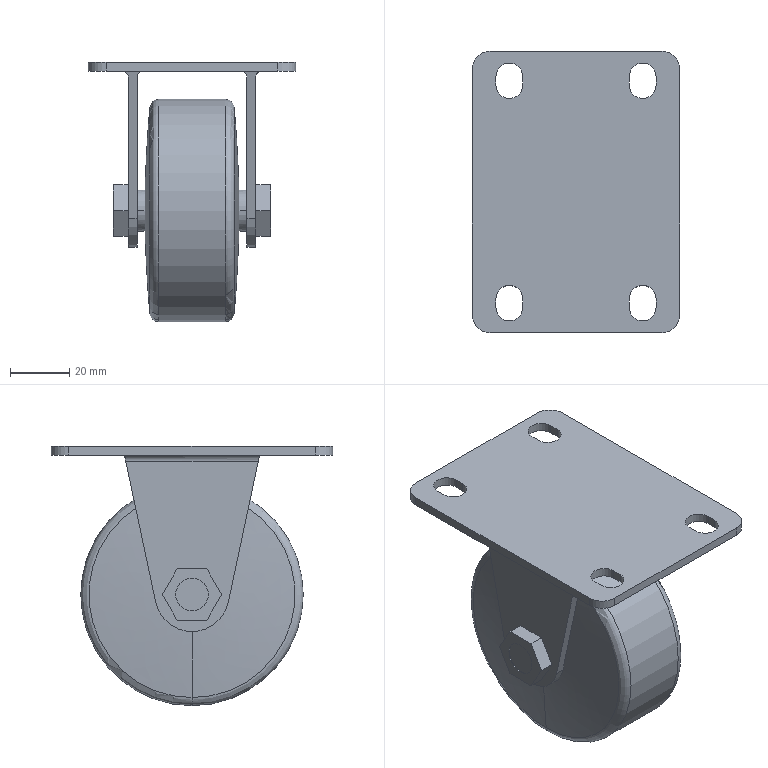Part | STEP file | Caster | 1 solid | 71 faces | box 70 x 95 x 87.5 mm | volume 164739 mm3 | plane 37 | cylinder 26 | other 4 | torus 4 | commonest cylinder face diameters 9 x8 4 x4 12 x4 14 x4 11.02 x2 25 x2